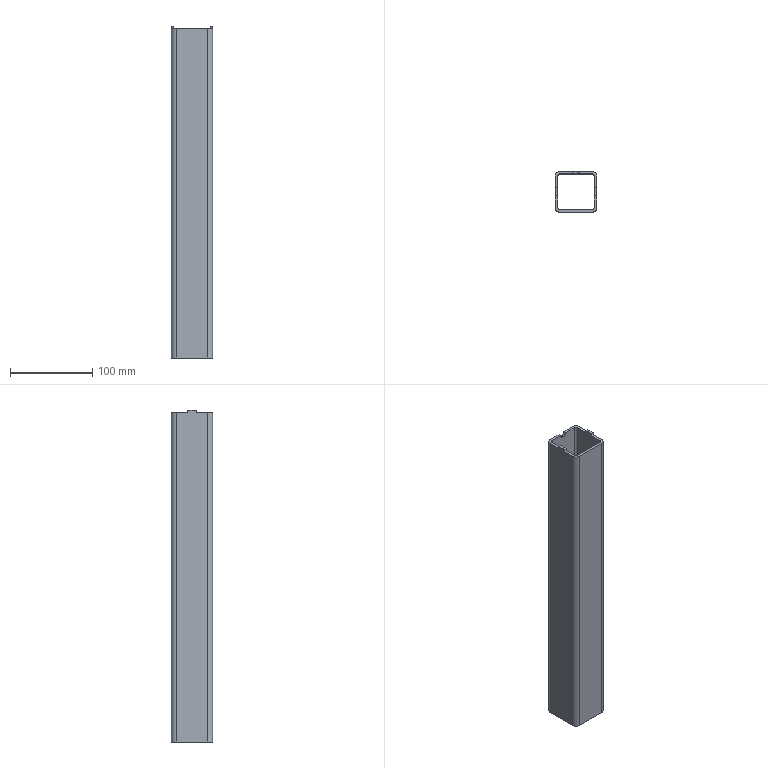Part | SolidWorks | features BaseBody 1 | 1 solid | 91 faces | box 50 x 50 x 403 mm | volume 216139 mm3 | plane 45 | spline 35 | cylinder 11 | commonest cylinder face diameters 6 x4 12 x4 8 x3